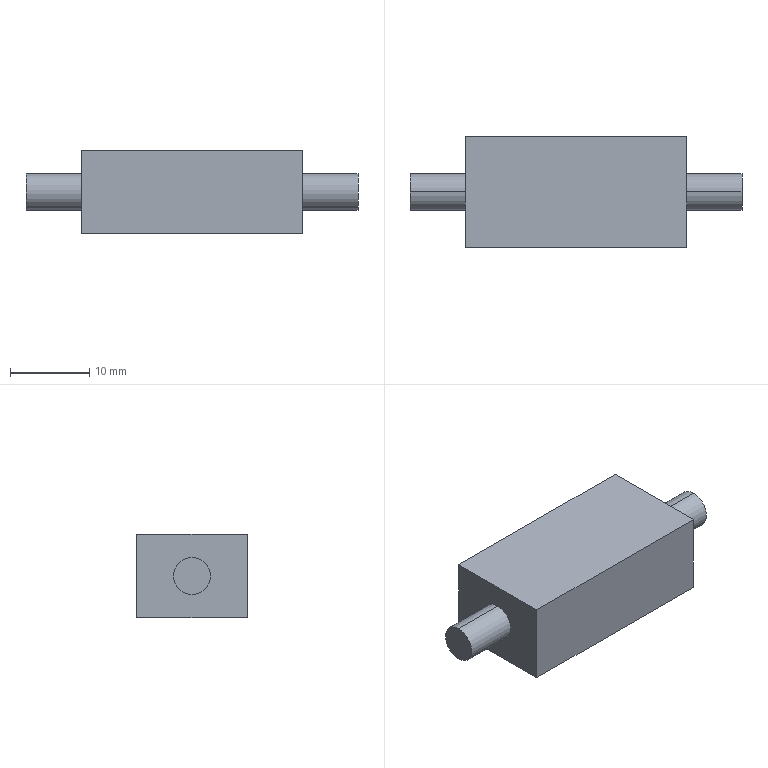Part | SolidWorks | features ICE 4, Extrusion 1, Scale 1 | 1 solid | 19 faces | box 42 x 14 x 10.5 mm | volume 3376 mm3 | plane 14 | cylinder 5 | commonest cylinder face diameters 4.665 x4 5.6 x1
STEP:
#1=CARTESIAN_POINT('',(21.,7.,-2.333));
#2=VERTEX_POINT('',#1);
#3=CARTESIAN_POINT('',(21.,7.,2.333));
#4=VERTEX_POINT('',#3);
#5=CARTESIAN_POINT('',(21.,7.,0.));
#6=DIRECTION('',(1.,0.,0.));
#7=DIRECTION('',(0.,0.,-1.));
#8=AXIS2_PLACEMENT_3D('',#5,#6,#7);
#9=CIRCLE('',#8,2.333);
#10=EDGE_CURVE('',#2,#4,#9,.T.);
#11=ORIENTED_EDGE('',*,*,#10,.F.);
#12=CARTESIAN_POINT('',(14.,7.,-2.333));
#13=VERTEX_POINT('',#12);
#14=CARTESIAN_POINT('',(21.,7.,-2.333));
#15=DIRECTION('',(-1.,0.,0.));
#16=VECTOR('',#15,1000.);
#17=LINE('',#14,#16);
#18=EDGE_CURVE('',#2,#13,#17,.T.);
#19=ORIENTED_EDGE('',*,*,#18,.T.);
#20=CARTESIAN_POINT('',(14.,7.,2.333));
#21=VERTEX_POINT('',#20);
#22=CARTESIAN_POINT('',(14.,7.,0.));
#23=DIRECTION('',(1.,0.,0.));
#24=DIRECTION('',(0.,0.,-1.));
#25=AXIS2_PLACEMENT_3D('',#22,#23,#24);
#26=CIRCLE('',#25,2.333);
#27=EDGE_CURVE('',#13,#21,#26,.T.);
#28=ORIENTED_EDGE('',*,*,#27,.T.);
#29=CARTESIAN_POINT('',(21.,7.,2.333));
#30=DIRECTION('',(-1.,0.,0.));
#31=VECTOR('',#30,1000.);
#32=LINE('',#29,#31);
#33=EDGE_CURVE('',#4,#21,#32,.T.);
#34=ORIENTED_EDGE('',*,*,#33,.F.);
#35=EDGE_LOOP('',(#11,#19,#28,#34));
#36=FACE_OUTER_BOUND('',#35,.T.);
#37=CARTESIAN_POINT('',(21.,7.,0.));
#38=DIRECTION('',(-1.,0.,0.));
#39=DIRECTION('',(0.,0.,1.));
#40=AXIS2_PLACEMENT_3D('',#37,#38,#39);
#41=CYLINDRICAL_SURFACE('',#40,2.333);
#42=ADVANCED_FACE('',(#36),#41,.T.);
#43=CARTESIAN_POINT('',(-21.,7.,2.333));
#44=VERTEX_POINT('',#43);
#45=CARTESIAN_POINT('',(-21.,7.,-2.333));
#46=VERTEX_POINT('',#45);
#47=CARTESIAN_POINT('',(-21.,7.,0.));
#48=DIRECTION('',(-1.,0.,0.));
#49=DIRECTION('',(0.,0.,1.));
#50=AXIS2_PLACEMENT_3D('',#47,#48,#49);
#51=CIRCLE('',#50,2.333);
#52=EDGE_CURVE('',#44,#46,#51,.T.);
#53=ORIENTED_EDGE('',*,*,#52,.F.);
#54=CARTESIAN_POINT('',(-14.,7.,2.333));
#55=VERTEX_POINT('',#54);
#56=CARTESIAN_POINT('',(-21.,7.,2.333));
#57=DIRECTION('',(1.,0.,0.));
#58=VECTOR('',#57,1000.);
#59=LINE('',#56,#58);
#60=EDGE_CURVE('',#44,#55,#59,.T.);
#61=ORIENTED_EDGE('',*,*,#60,.T.);
#62=CARTESIAN_POINT('',(-14.,7.,-2.333));
#63=VERTEX_POINT('',#62);
#64=CARTESIAN_POINT('',(-14.,7.,0.));
#65=DIRECTION('',(-1.,0.,0.));
#66=DIRECTION('',(0.,0.,1.));
#67=AXIS2_PLACEMENT_3D('',#64,#65,#66);
#68=CIRCLE('',#67,2.333);
#69=EDGE_CURVE('',#55,#63,#68,.T.);
#70=ORIENTED_EDGE('',*,*,#69,.T.);
#71=CARTESIAN_POINT('',(-21.,7.,-2.333));
#72=DIRECTION('',(1.,0.,0.));
#73=VECTOR('',#72,1000.);
#74=LINE('',#71,#73);
#75=EDGE_CURVE('',#46,#63,#74,.T.);
#76=ORIENTED_EDGE('',*,*,#75,.F.);
#77=EDGE_LOOP('',(#53,#61,#70,#76));
#78=FACE_OUTER_BOUND('',#77,.T.);
#79=CARTESIAN_POINT('',(-21.,7.,0.));
#80=DIRECTION('',(1.,0.,0.));
#81=DIRECTION('',(0.,0.,-1.));
#82=AXIS2_PLACEMENT_3D('',#79,#80,#81);
#83=CYLINDRICAL_SURFACE('',#82,2.333);
#84=ADVANCED_FACE('',(#78),#83,.T.);
#85=CARTESIAN_POINT('',(-12.261,7.,2.8));
#86=VERTEX_POINT('',#85);
#87=CARTESIAN_POINT('',(12.261,7.,2.8));
#88=VERTEX_POINT('',#87);
#89=CARTESIAN_POINT('',(20.181,7.,2.8));
#90=DIRECTION('',(1.,0.,0.));
#91=VECTOR('',#90,1000.);
#92=LINE('',#89,#91);
#93=EDGE_CURVE('',#86,#88,#92,.T.);
#94=ORIENTED_EDGE('',*,*,#93,.F.);
#95=CARTESIAN_POINT('',(-12.261,7.,3.731));
#96=VERTEX_POINT('',#95);
#97=CARTESIAN_POINT('',(-12.261,7.,3.731));
#98=DIRECTION('',(0.,0.,1.));
#99=VECTOR('',#98,1000.);
#100=LINE('',#97,#99);
#101=EDGE_CURVE('',#86,#96,#100,.T.);
#102=ORIENTED_EDGE('',*,*,#101,.T.);
#103=CARTESIAN_POINT('',(12.261,7.,3.731));
#104=VERTEX_POINT('',#103);
#105=CARTESIAN_POINT('',(-12.261,7.,3.731));
#106=DIRECTION('',(1.,0.,0.));
#107=VECTOR('',#106,1000.);
#108=LINE('',#105,#107);
#109=EDGE_CURVE('',#96,#104,#108,.T.);
#110=ORIENTED_EDGE('',*,*,#109,.T.);
#111=CARTESIAN_POINT('',(12.261,7.,3.731));
#112=DIRECTION('',(0.,0.,-1.));
#113=VECTOR('',#112,1000.);
#114=LINE('',#111,#113);
#115=EDGE_CURVE('',#104,#88,#114,.T.);
#116=ORIENTED_EDGE('',*,*,#115,.T.);
#117=EDGE_LOOP('',(#94,#102,#110,#116));
#118=FACE_OUTER_BOUND('',#117,.T.);
#119=CARTESIAN_POINT('',(0.,7.,0.));
#120=DIRECTION('',(0.,-1.,0.));
#121=DIRECTION('',(0.,0.,-1.));
#122=AXIS2_PLACEMENT_3D('',#119,#120,#121);
#123=PLANE('',#122);
#124=ADVANCED_FACE('',(#118),#123,.F.);
#125=CARTESIAN_POINT('',(12.261,7.,-2.8));
#126=VERTEX_POINT('',#125);
#127=CARTESIAN_POINT('',(-12.261,7.,-2.8));
#128=VERTEX_POINT('',#127);
#129=CARTESIAN_POINT('',(20.181,7.,-2.8));
#130=DIRECTION('',(-1.,0.,0.));
#131=VECTOR('',#130,1000.);
#132=LINE('',#129,#131);
#133=EDGE_CURVE('',#126,#128,#132,.T.);
#134=ORIENTED_EDGE('',*,*,#133,.F.);
#135=CARTESIAN_POINT('',(12.261,7.,-3.731));
#136=VERTEX_POINT('',#135);
#137=CARTESIAN_POINT('',(12.261,7.,3.731));
#138=DIRECTION('',(0.,0.,-1.));
#139=VECTOR('',#138,1000.);
#140=LINE('',#137,#139);
#141=EDGE_CURVE('',#126,#136,#140,.T.);
#142=ORIENTED_EDGE('',*,*,#141,.T.);
#143=CARTESIAN_POINT('',(-12.261,7.,-3.731));
#144=VERTEX_POINT('',#143);
#145=CARTESIAN_POINT('',(-12.261,7.,-3.731));
#146=DIRECTION('',(-1.,0.,0.));
#147=VECTOR('',#146,1000.);
#148=LINE('',#145,#147);
#149=EDGE_CURVE('',#136,#144,#148,.T.);
#150=ORIENTED_EDGE('',*,*,#149,.T.);
#151=CARTESIAN_POINT('',(-12.261,7.,3.731));
#152=DIRECTION('',(0.,0.,1.));
#153=VECTOR('',#152,1000.);
#154=LINE('',#151,#153);
#155=EDGE_CURVE('',#144,#128,#154,.T.);
#156=ORIENTED_EDGE('',*,*,#155,.T.);
#157=EDGE_LOOP('',(#134,#142,#150,#156));
#158=FACE_OUTER_BOUND('',#157,.T.);
#159=CARTESIAN_POINT('',(0.,7.,0.));
#160=DIRECTION('',(0.,-1.,0.));
#161=DIRECTION('',(0.,0.,-1.));
#162=AXIS2_PLACEMENT_3D('',#159,#160,#161);
#163=PLANE('',#162);
#164=ADVANCED_FACE('',(#158),#163,.F.);
#165=CARTESIAN_POINT('',(14.,7.,0.));
#166=DIRECTION('',(1.,0.,0.));
#167=DIRECTION('',(0.,0.,-1.));
#168=AXIS2_PLACEMENT_3D('',#165,#166,#167);
#169=CIRCLE('',#168,2.333);
#170=EDGE_CURVE('',#21,#13,#169,.T.);
#171=ORIENTED_EDGE('',*,*,#170,.F.);
#172=ORIENTED_EDGE('',*,*,#27,.F.);
#173=EDGE_LOOP('',(#171,#172));
#174=FACE_BOUND('',#173,.T.);
#175=CARTESIAN_POINT('',(14.,0.,5.25));
#176=VERTEX_POINT('',#175);
#177=CARTESIAN_POINT('',(14.,0.,-5.25));
#178=VERTEX_POINT('',#177);
#179=CARTESIAN_POINT('',(14.,0.,-5.25));
#180=DIRECTION('',(0.,0.,-1.));
#181=VECTOR('',#180,1000.);
#182=LINE('',#179,#181);
#183=EDGE_CURVE('',#176,#178,#182,.T.);
#184=ORIENTED_EDGE('',*,*,#183,.T.);
#185=CARTESIAN_POINT('',(14.,14.,-5.25));
#186=VERTEX_POINT('',#185);
#187=CARTESIAN_POINT('',(14.,14.,-5.25));
#188=DIRECTION('',(0.,-1.,0.));
#189=VECTOR('',#188,1000.);
#190=LINE('',#187,#189);
#191=EDGE_CURVE('',#186,#178,#190,.T.);
#192=ORIENTED_EDGE('',*,*,#191,.F.);
#193=CARTESIAN_POINT('',(14.,14.,5.25));
#194=VERTEX_POINT('',#193);
#195=CARTESIAN_POINT('',(14.,14.,-5.25));
#196=DIRECTION('',(0.,0.,-1.));
#197=VECTOR('',#196,1000.);
#198=LINE('',#195,#197);
#199=EDGE_CURVE('',#194,#186,#198,.T.);
#200=ORIENTED_EDGE('',*,*,#199,.F.);
#201=CARTESIAN_POINT('',(14.,14.,5.25));
#202=DIRECTION('',(0.,-1.,0.));
#203=VECTOR('',#202,1000.);
#204=LINE('',#201,#203);
#205=EDGE_CURVE('',#194,#176,#204,.T.);
#206=ORIENTED_EDGE('',*,*,#205,.T.);
#207=EDGE_LOOP('',(#184,#192,#200,#206));
#208=FACE_OUTER_BOUND('',#207,.T.);
#209=CARTESIAN_POINT('',(14.,14.,-5.25));
#210=DIRECTION('',(-1.,0.,0.));
#211=DIRECTION('',(0.,0.,1.));
#212=AXIS2_PLACEMENT_3D('',#209,#210,#211);
#213=PLANE('',#212);
#214=ADVANCED_FACE('',(#174,#208),#213,.F.);
#215=CARTESIAN_POINT('',(-14.,0.,-5.25));
#216=VERTEX_POINT('',#215);
#217=CARTESIAN_POINT('',(-14.,0.,-5.25));
#218=DIRECTION('',(-1.,0.,0.));
#219=VECTOR('',#218,1000.);
#220=LINE('',#217,#219);
#221=EDGE_CURVE('',#178,#216,#220,.T.);
#222=ORIENTED_EDGE('',*,*,#221,.T.);
#223=CARTESIAN_POINT('',(-14.,14.,-5.25));
#224=VERTEX_POINT('',#223);
#225=CARTESIAN_POINT('',(-14.,14.,-5.25));
#226=DIRECTION('',(0.,-1.,0.));
#227=VECTOR('',#226,1000.);
#228=LINE('',#225,#227);
#229=EDGE_CURVE('',#224,#216,#228,.T.);
#230=ORIENTED_EDGE('',*,*,#229,.F.);
#231=CARTESIAN_POINT('',(-14.,14.,-5.25));
#232=DIRECTION('',(-1.,0.,0.));
#233=VECTOR('',#232,1000.);
#234=LINE('',#231,#233);
#235=EDGE_CURVE('',#186,#224,#234,.T.);
#236=ORIENTED_EDGE('',*,*,#235,.F.);
#237=ORIENTED_EDGE('',*,*,#191,.T.);
#238=EDGE_LOOP('',(#222,#230,#236,#237));
#239=FACE_OUTER_BOUND('',#238,.T.);
#240=CARTESIAN_POINT('',(-14.,14.,-5.25));
#241=DIRECTION('',(0.,0.,1.));
#242=DIRECTION('',(1.,0.,0.));
#243=AXIS2_PLACEMENT_3D('',#240,#241,#242);
#244=PLANE('',#243);
#245=ADVANCED_FACE('',(#239),#244,.F.);
#246=CARTESIAN_POINT('',(-14.,7.,0.));
#247=DIRECTION('',(-1.,0.,0.));
#248=DIRECTION('',(0.,0.,1.));
#249=AXIS2_PLACEMENT_3D('',#246,#247,#248);
#250=CIRCLE('',#249,2.333);
#251=EDGE_CURVE('',#63,#55,#250,.T.);
#252=ORIENTED_EDGE('',*,*,#251,.F.);
#253=ORIENTED_EDGE('',*,*,#69,.F.);
#254=EDGE_LOOP('',(#252,#253));
#255=FACE_BOUND('',#254,.T.);
#256=CARTESIAN_POINT('',(-14.,0.,5.25));
#257=VERTEX_POINT('',#256);
#258=CARTESIAN_POINT('',(-14.,0.,-5.25));
#259=DIRECTION('',(0.,0.,1.));
#260=VECTOR('',#259,1000.);
#261=LINE('',#258,#260);
#262=EDGE_CURVE('',#216,#257,#261,.T.);
#263=ORIENTED_EDGE('',*,*,#262,.T.);
#264=CARTESIAN_POINT('',(-14.,14.,5.25));
#265=VERTEX_POINT('',#264);
#266=CARTESIAN_POINT('',(-14.,14.,5.25));
#267=DIRECTION('',(0.,-1.,0.));
#268=VECTOR('',#267,1000.);
#269=LINE('',#266,#268);
#270=EDGE_CURVE('',#265,#257,#269,.T.);
#271=ORIENTED_EDGE('',*,*,#270,.F.);
#272=CARTESIAN_POINT('',(-14.,14.,-5.25));
#273=DIRECTION('',(0.,0.,1.));
#274=VECTOR('',#273,1000.);
#275=LINE('',#272,#274);
#276=EDGE_CURVE('',#224,#265,#275,.T.);
#277=ORIENTED_EDGE('',*,*,#276,.F.);
#278=ORIENTED_EDGE('',*,*,#229,.T.);
#279=EDGE_LOOP('',(#263,#271,#277,#278));
#280=FACE_OUTER_BOUND('',#279,.T.);
#281=CARTESIAN_POINT('',(-14.,14.,-5.25));
#282=DIRECTION('',(1.,0.,0.));
#283=DIRECTION('',(0.,0.,-1.));
#284=AXIS2_PLACEMENT_3D('',#281,#282,#283);
#285=PLANE('',#284);
#286=ADVANCED_FACE('',(#255,#280),#285,.F.);
#287=CARTESIAN_POINT('',(-14.,0.,5.25));
#288=DIRECTION('',(1.,0.,0.));
#289=VECTOR('',#288,1000.);
#290=LINE('',#287,#289);
#291=EDGE_CURVE('',#257,#176,#290,.T.);
#292=ORIENTED_EDGE('',*,*,#291,.T.);
#293=ORIENTED_EDGE('',*,*,#205,.F.);
#294=CARTESIAN_POINT('',(-14.,14.,5.25));
#295=DIRECTION('',(1.,0.,0.));
#296=VECTOR('',#295,1000.);
#297=LINE('',#294,#296);
#298=EDGE_CURVE('',#265,#194,#297,.T.);
#299=ORIENTED_EDGE('',*,*,#298,.F.);
#300=ORIENTED_EDGE('',*,*,#270,.T.);
#301=EDGE_LOOP('',(#292,#293,#299,#300));
#302=FACE_OUTER_BOUND('',#301,.T.);
#303=CARTESIAN_POINT('',(-14.,14.,5.25));
#304=DIRECTION('',(0.,0.,-1.));
#305=DIRECTION('',(-1.,0.,0.));
#306=AXIS2_PLACEMENT_3D('',#303,#304,#305);
#307=PLANE('',#306);
#308=ADVANCED_FACE('',(#302),#307,.F.);
#309=CARTESIAN_POINT('',(12.261,14.,3.731));
#310=VERTEX_POINT('',#309);
#311=CARTESIAN_POINT('',(12.261,14.,-3.731));
#312=VERTEX_POINT('',#311);
#313=CARTESIAN_POINT('',(12.261,14.,3.731));
#314=DIRECTION('',(0.,0.,-1.));
#315=VECTOR('',#314,1000.);
#316=LINE('',#313,#315);
#317=EDGE_CURVE('',#310,#312,#316,.T.);
#318=ORIENTED_EDGE('',*,*,#317,.F.);
#319=CARTESIAN_POINT('',(-12.261,14.,3.731));
#320=VERTEX_POINT('',#319);
#321=CARTESIAN_POINT('',(-12.261,14.,3.731));
#322=DIRECTION('',(1.,0.,0.));
#323=VECTOR('',#322,1000.);
#324=LINE('',#321,#323);
#325=EDGE_CURVE('',#320,#310,#324,.T.);
#326=ORIENTED_EDGE('',*,*,#325,.F.);
#327=CARTESIAN_POINT('',(-12.261,14.,-3.731));
#328=VERTEX_POINT('',#327);
#329=CARTESIAN_POINT('',(-12.261,14.,3.731));
#330=DIRECTION('',(0.,0.,1.));
#331=VECTOR('',#330,1000.);
#332=LINE('',#329,#331);
#333=EDGE_CURVE('',#328,#320,#332,.T.);
#334=ORIENTED_EDGE('',*,*,#333,.F.);
#335=CARTESIAN_POINT('',(-12.261,14.,-3.731));
#336=DIRECTION('',(-1.,0.,0.));
#337=VECTOR('',#336,1000.);
#338=LINE('',#335,#337);
#339=EDGE_CURVE('',#312,#328,#338,.T.);
#340=ORIENTED_EDGE('',*,*,#339,.F.);
#341=EDGE_LOOP('',(#318,#326,#334,#340));
#342=FACE_BOUND('',#341,.T.);
#343=ORIENTED_EDGE('',*,*,#199,.T.);
#344=ORIENTED_EDGE('',*,*,#235,.T.);
#345=ORIENTED_EDGE('',*,*,#276,.T.);
#346=ORIENTED_EDGE('',*,*,#298,.T.);
#347=EDGE_LOOP('',(#343,#344,#345,#346));
#348=FACE_OUTER_BOUND('',#347,.T.);
#349=CARTESIAN_POINT('',(0.,14.,0.));
#350=DIRECTION('',(0.,1.,0.));
#351=DIRECTION('',(0.,0.,1.));
#352=AXIS2_PLACEMENT_3D('',#349,#350,#351);
#353=PLANE('',#352);
#354=ADVANCED_FACE('',(#342,#348),#353,.T.);
#355=ORIENTED_EDGE('',*,*,#183,.F.);
#356=ORIENTED_EDGE('',*,*,#291,.F.);
#357=ORIENTED_EDGE('',*,*,#262,.F.);
#358=ORIENTED_EDGE('',*,*,#221,.F.);
#359=EDGE_LOOP('',(#355,#356,#357,#358));
#360=FACE_OUTER_BOUND('',#359,.T.);
#361=CARTESIAN_POINT('',(0.,0.,0.));
#362=DIRECTION('',(0.,1.,0.));
#363=DIRECTION('',(0.,0.,1.));
#364=AXIS2_PLACEMENT_3D('',#361,#362,#363);
#365=PLANE('',#364);
#366=ADVANCED_FACE('',(#360),#365,.F.);
#367=CARTESIAN_POINT('',(12.261,7.,0.));
#368=DIRECTION('',(1.,0.,0.));
#369=DIRECTION('',(0.,0.,-1.));
#370=AXIS2_PLACEMENT_3D('',#367,#368,#369);
#371=CIRCLE('',#370,2.8);
#372=EDGE_CURVE('',#126,#88,#371,.T.);
#373=ORIENTED_EDGE('',*,*,#372,.T.);
#374=ORIENTED_EDGE('',*,*,#115,.F.);
#375=CARTESIAN_POINT('',(12.261,7.,3.731));
#376=DIRECTION('',(0.,1.,0.));
#377=VECTOR('',#376,1000.);
#378=LINE('',#375,#377);
#379=EDGE_CURVE('',#104,#310,#378,.T.);
#380=ORIENTED_EDGE('',*,*,#379,.T.);
#381=ORIENTED_EDGE('',*,*,#317,.T.);
#382=CARTESIAN_POINT('',(12.261,7.,-3.731));
#383=DIRECTION('',(0.,1.,0.));
#384=VECTOR('',#383,1000.);
#385=LINE('',#382,#384);
#386=EDGE_CURVE('',#136,#312,#385,.T.);
#387=ORIENTED_EDGE('',*,*,#386,.F.);
#388=ORIENTED_EDGE('',*,*,#141,.F.);
#389=EDGE_LOOP('',(#373,#374,#380,#381,#387,#388));
#390=FACE_OUTER_BOUND('',#389,.T.);
#391=CARTESIAN_POINT('',(12.261,7.,3.731));
#392=DIRECTION('',(1.,0.,0.));
#393=DIRECTION('',(0.,0.,-1.));
#394=AXIS2_PLACEMENT_3D('',#391,#392,#393);
#395=PLANE('',#394);
#396=ADVANCED_FACE('',(#390),#395,.F.);
#397=ORIENTED_EDGE('',*,*,#325,.T.);
#398=ORIENTED_EDGE('',*,*,#379,.F.);
#399=ORIENTED_EDGE('',*,*,#109,.F.);
#400=CARTESIAN_POINT('',(-12.261,7.,3.731));
#401=DIRECTION('',(0.,1.,0.));
#402=VECTOR('',#401,1000.);
#403=LINE('',#400,#402);
#404=EDGE_CURVE('',#96,#320,#403,.T.);
#405=ORIENTED_EDGE('',*,*,#404,.T.);
#406=EDGE_LOOP('',(#397,#398,#399,#405));
#407=FACE_OUTER_BOUND('',#406,.T.);
#408=CARTESIAN_POINT('',(-12.261,7.,3.731));
#409=DIRECTION('',(0.,0.,1.));
#410=DIRECTION('',(1.,0.,0.));
#411=AXIS2_PLACEMENT_3D('',#408,#409,#410);
#412=PLANE('',#411);
#413=ADVANCED_FACE('',(#407),#412,.F.);
#414=CARTESIAN_POINT('',(-12.261,7.,0.));
#415=DIRECTION('',(1.,0.,0.));
#416=DIRECTION('',(0.,0.,-1.));
#417=AXIS2_PLACEMENT_3D('',#414,#415,#416);
#418=CIRCLE('',#417,2.8);
#419=EDGE_CURVE('',#128,#86,#418,.T.);
#420=ORIENTED_EDGE('',*,*,#419,.F.);
#421=ORIENTED_EDGE('',*,*,#155,.F.);
#422=CARTESIAN_POINT('',(-12.261,7.,-3.731));
#423=DIRECTION('',(0.,1.,0.));
#424=VECTOR('',#423,1000.);
#425=LINE('',#422,#424);
#426=EDGE_CURVE('',#144,#328,#425,.T.);
#427=ORIENTED_EDGE('',*,*,#426,.T.);
#428=ORIENTED_EDGE('',*,*,#333,.T.);
#429=ORIENTED_EDGE('',*,*,#404,.F.);
#430=ORIENTED_EDGE('',*,*,#101,.F.);
#431=EDGE_LOOP('',(#420,#421,#427,#428,#429,#430));
#432=FACE_OUTER_BOUND('',#431,.T.);
#433=CARTESIAN_POINT('',(-12.261,7.,3.731));
#434=DIRECTION('',(-1.,0.,0.));
#435=DIRECTION('',(0.,0.,1.));
#436=AXIS2_PLACEMENT_3D('',#433,#434,#435);
#437=PLANE('',#436);
#438=ADVANCED_FACE('',(#432),#437,.F.);
#439=ORIENTED_EDGE('',*,*,#339,.T.);
#440=ORIENTED_EDGE('',*,*,#426,.F.);
#441=ORIENTED_EDGE('',*,*,#149,.F.);
#442=ORIENTED_EDGE('',*,*,#386,.T.);
#443=EDGE_LOOP('',(#439,#440,#441,#442));
#444=FACE_OUTER_BOUND('',#443,.T.);
#445=CARTESIAN_POINT('',(-12.261,7.,-3.731));
#446=DIRECTION('',(0.,0.,-1.));
#447=DIRECTION('',(-1.,0.,0.));
#448=AXIS2_PLACEMENT_3D('',#445,#446,#447);
#449=PLANE('',#448);
#450=ADVANCED_FACE('',(#444),#449,.F.);
#451=ORIENTED_EDGE('',*,*,#419,.T.);
#452=ORIENTED_EDGE('',*,*,#93,.T.);
#453=ORIENTED_EDGE('',*,*,#372,.F.);
#454=ORIENTED_EDGE('',*,*,#133,.T.);
#455=EDGE_LOOP('',(#451,#452,#453,#454));
#456=FACE_OUTER_BOUND('',#455,.T.);
#457=CARTESIAN_POINT('',(20.181,7.,0.));
#458=DIRECTION('',(-1.,0.,0.));
#459=DIRECTION('',(0.,0.,1.));
#460=AXIS2_PLACEMENT_3D('',#457,#458,#459);
#461=CYLINDRICAL_SURFACE('',#460,2.8);
#462=ADVANCED_FACE('',(#456),#461,.T.);
#463=ORIENTED_EDGE('',*,*,#60,.F.);
#464=CARTESIAN_POINT('',(-21.,7.,0.));
#465=DIRECTION('',(-1.,0.,0.));
#466=DIRECTION('',(0.,0.,1.));
#467=AXIS2_PLACEMENT_3D('',#464,#465,#466);
#468=CIRCLE('',#467,2.333);
#469=EDGE_CURVE('',#46,#44,#468,.T.);
#470=ORIENTED_EDGE('',*,*,#469,.F.);
#471=ORIENTED_EDGE('',*,*,#75,.T.);
#472=ORIENTED_EDGE('',*,*,#251,.T.);
#473=EDGE_LOOP('',(#463,#470,#471,#472));
#474=FACE_OUTER_BOUND('',#473,.T.);
#475=CARTESIAN_POINT('',(-21.,7.,0.));
#476=DIRECTION('',(1.,0.,0.));
#477=DIRECTION('',(0.,0.,-1.));
#478=AXIS2_PLACEMENT_3D('',#475,#476,#477);
#479=CYLINDRICAL_SURFACE('',#478,2.333);
#480=ADVANCED_FACE('',(#474),#479,.T.);
#481=ORIENTED_EDGE('',*,*,#469,.T.);
#482=ORIENTED_EDGE('',*,*,#52,.T.);
#483=EDGE_LOOP('',(#481,#482));
#484=FACE_OUTER_BOUND('',#483,.T.);
#485=CARTESIAN_POINT('',(-21.,7.,0.));
#486=DIRECTION('',(-1.,0.,0.));
#487=DIRECTION('',(0.,0.,1.));
#488=AXIS2_PLACEMENT_3D('',#485,#486,#487);
#489=PLANE('',#488);
#490=ADVANCED_FACE('',(#484),#489,.T.);
#491=ORIENTED_EDGE('',*,*,#18,.F.);
#492=CARTESIAN_POINT('',(21.,7.,0.));
#493=DIRECTION('',(1.,0.,0.));
#494=DIRECTION('',(0.,0.,-1.));
#495=AXIS2_PLACEMENT_3D('',#492,#493,#494);
#496=CIRCLE('',#495,2.333);
#497=EDGE_CURVE('',#4,#2,#496,.T.);
#498=ORIENTED_EDGE('',*,*,#497,.F.);
#499=ORIENTED_EDGE('',*,*,#33,.T.);
#500=ORIENTED_EDGE('',*,*,#170,.T.);
#501=EDGE_LOOP('',(#491,#498,#499,#500));
#502=FACE_OUTER_BOUND('',#501,.T.);
#503=CARTESIAN_POINT('',(21.,7.,0.));
#504=DIRECTION('',(-1.,0.,0.));
#505=DIRECTION('',(0.,0.,1.));
#506=AXIS2_PLACEMENT_3D('',#503,#504,#505);
#507=CYLINDRICAL_SURFACE('',#506,2.333);
#508=ADVANCED_FACE('',(#502),#507,.T.);
#509=ORIENTED_EDGE('',*,*,#497,.T.);
#510=ORIENTED_EDGE('',*,*,#10,.T.);
#511=EDGE_LOOP('',(#509,#510));
#512=FACE_OUTER_BOUND('',#511,.T.);
#513=CARTESIAN_POINT('',(21.,7.,0.));
#514=DIRECTION('',(1.,0.,0.));
#515=DIRECTION('',(0.,0.,-1.));
#516=AXIS2_PLACEMENT_3D('',#513,#514,#515);
#517=PLANE('',#516);
#518=ADVANCED_FACE('',(#512),#517,.T.);
#519=CLOSED_SHELL('',(#42,#84,#124,#164,#214,#245,#286,#308,#354,#366,#396,#413,#438,#450,#462,#480,#490,#508,#518));
#520=MANIFOLD_SOLID_BREP('',#519);
#521=CARTESIAN_POINT('',(0.,0.,0.));
#522=DIRECTION('',(0.,0.,1.));
#523=DIRECTION('',(1.,0.,0.));
#524=AXIS2_PLACEMENT_3D('',#521,#522,#523);
#525=(LENGTH_UNIT()NAMED_UNIT(*)SI_UNIT(.MILLI.,.METRE.));
#526=UNCERTAINTY_MEASURE_WITH_UNIT(LENGTH_MEASURE(0.00001),#525,'','');
#527=(NAMED_UNIT(*)PLANE_ANGLE_UNIT()SI_UNIT($,.RADIAN.));
#528=(NAMED_UNIT(*)SI_UNIT($,.STERADIAN.)SOLID_ANGLE_UNIT());
#529=(GEOMETRIC_REPRESENTATION_CONTEXT(3)GLOBAL_UNCERTAINTY_ASSIGNED_CONTEXT((#526))GLOBAL_UNIT_ASSIGNED_CONTEXT((#525,#527,#528))REPRESENTATION_CONTEXT('',''));
#530=ADVANCED_BREP_SHAPE_REPRESENTATION('',(#520,#524),#529);